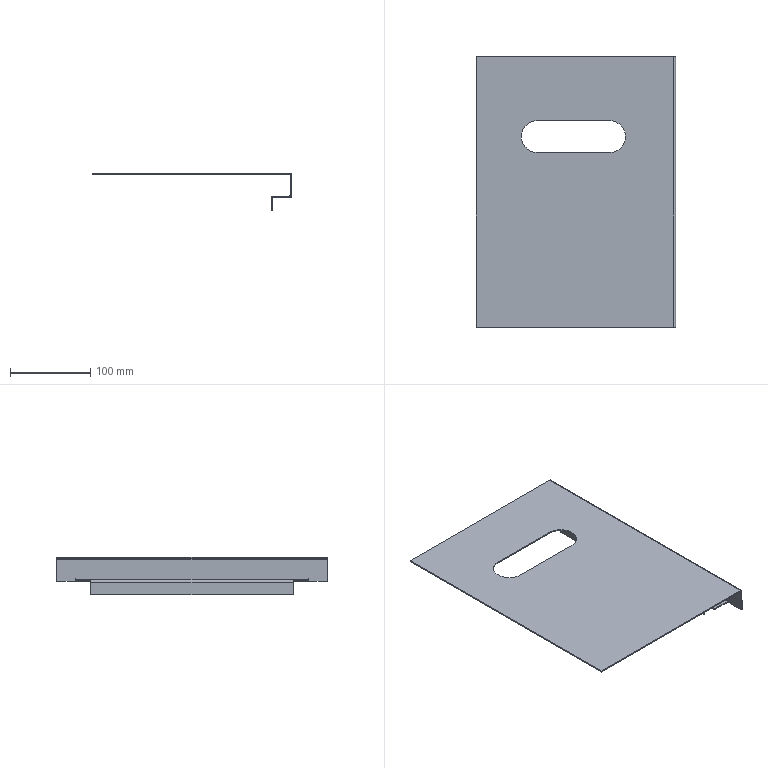Part | SolidWorks | features EdgeFlange 3, Cut 1, FlatPattern 1, SMBaseFlange 1, SheetMetal 1 | 1 solid | 51 faces | box 248.5 x 337 x 47 mm | volume 148406 mm3 | plane 42 | cylinder 9 | commonest cylinder face diameters 2 x3 5 x3 40 x3
STEP:
#1=CARTESIAN_POINT('',(56.,237.5,0.));
#2=VERTEX_POINT('',#1);
#3=CARTESIAN_POINT('',(76.,257.5,0.));
#4=VERTEX_POINT('',#3);
#5=CARTESIAN_POINT('',(76.,237.5,0.));
#6=DIRECTION('',(0.,0.,-1.));
#7=DIRECTION('',(-1.,0.,0.));
#8=AXIS2_PLACEMENT_3D('',#5,#6,#7);
#9=CIRCLE('',#8,20.);
#10=EDGE_CURVE('',#2,#4,#9,.T.);
#11=ORIENTED_EDGE('',*,*,#10,.F.);
#12=CARTESIAN_POINT('',(56.,237.5,-1.5));
#13=VERTEX_POINT('',#12);
#14=CARTESIAN_POINT('',(56.,237.5,0.));
#15=DIRECTION('',(0.,0.,-1.));
#16=VECTOR('',#15,1000.);
#17=LINE('',#14,#16);
#18=EDGE_CURVE('',#2,#13,#17,.T.);
#19=ORIENTED_EDGE('',*,*,#18,.T.);
#20=CARTESIAN_POINT('',(76.,257.5,-1.5));
#21=VERTEX_POINT('',#20);
#22=CARTESIAN_POINT('',(76.,237.5,-1.5));
#23=DIRECTION('',(0.,0.,-1.));
#24=DIRECTION('',(-1.,0.,0.));
#25=AXIS2_PLACEMENT_3D('',#22,#23,#24);
#26=CIRCLE('',#25,20.);
#27=EDGE_CURVE('',#13,#21,#26,.T.);
#28=ORIENTED_EDGE('',*,*,#27,.T.);
#29=CARTESIAN_POINT('',(76.,257.5,0.));
#30=DIRECTION('',(0.,0.,-1.));
#31=VECTOR('',#30,1000.);
#32=LINE('',#29,#31);
#33=EDGE_CURVE('',#4,#21,#32,.T.);
#34=ORIENTED_EDGE('',*,*,#33,.F.);
#35=EDGE_LOOP('',(#11,#19,#28,#34));
#36=FACE_OUTER_BOUND('',#35,.T.);
#37=CARTESIAN_POINT('',(76.,237.5,0.));
#38=DIRECTION('',(0.,0.,-1.));
#39=DIRECTION('',(-1.,0.,0.));
#40=AXIS2_PLACEMENT_3D('',#37,#38,#39);
#41=CYLINDRICAL_SURFACE('',#40,20.);
#42=ADVANCED_FACE('',(#36),#41,.F.);
#43=CARTESIAN_POINT('',(226.75,295.75,-30.));
#44=VERTEX_POINT('',#43);
#45=CARTESIAN_POINT('',(226.75,295.,-30.));
#46=VERTEX_POINT('',#45);
#47=CARTESIAN_POINT('',(226.75,295.75,-30.));
#48=DIRECTION('',(0.,-1.,0.));
#49=VECTOR('',#48,1000.);
#50=LINE('',#47,#49);
#51=EDGE_CURVE('',#44,#46,#50,.T.);
#52=ORIENTED_EDGE('',*,*,#51,.F.);
#53=CARTESIAN_POINT('',(223.5,295.75,-30.));
#54=VERTEX_POINT('',#53);
#55=CARTESIAN_POINT('',(223.5,295.75,-30.));
#56=DIRECTION('',(1.,0.,0.));
#57=VECTOR('',#56,1000.);
#58=LINE('',#55,#57);
#59=EDGE_CURVE('',#54,#44,#58,.T.);
#60=ORIENTED_EDGE('',*,*,#59,.F.);
#61=CARTESIAN_POINT('',(223.5,313.5,-30.));
#62=VERTEX_POINT('',#61);
#63=CARTESIAN_POINT('',(223.5,23.5,-30.));
#64=DIRECTION('',(0.,-1.,0.));
#65=VECTOR('',#64,1000.);
#66=LINE('',#63,#65);
#67=EDGE_CURVE('',#62,#54,#66,.T.);
#68=ORIENTED_EDGE('',*,*,#67,.F.);
#69=CARTESIAN_POINT('',(246.,313.5,-30.));
#70=VERTEX_POINT('',#69);
#71=CARTESIAN_POINT('',(223.5,313.5,-30.));
#72=DIRECTION('',(-1.,0.,0.));
#73=VECTOR('',#72,1000.);
#74=LINE('',#71,#73);
#75=EDGE_CURVE('',#70,#62,#74,.T.);
#76=ORIENTED_EDGE('',*,*,#75,.F.);
#77=CARTESIAN_POINT('',(246.,23.5,-30.));
#78=VERTEX_POINT('',#77);
#79=CARTESIAN_POINT('',(246.,0.,-30.));
#80=DIRECTION('',(0.,-1.,0.));
#81=VECTOR('',#80,1000.);
#82=LINE('',#79,#81);
#83=EDGE_CURVE('',#70,#78,#82,.T.);
#84=ORIENTED_EDGE('',*,*,#83,.T.);
#85=CARTESIAN_POINT('',(223.5,23.5,-30.));
#86=VERTEX_POINT('',#85);
#87=CARTESIAN_POINT('',(247.,23.5,-30.));
#88=DIRECTION('',(1.,0.,0.));
#89=VECTOR('',#88,1000.);
#90=LINE('',#87,#89);
#91=EDGE_CURVE('',#86,#78,#90,.T.);
#92=ORIENTED_EDGE('',*,*,#91,.F.);
#93=CARTESIAN_POINT('',(223.5,41.25,-30.));
#94=VERTEX_POINT('',#93);
#95=CARTESIAN_POINT('',(223.5,23.5,-30.));
#96=DIRECTION('',(0.,-1.,0.));
#97=VECTOR('',#96,1000.);
#98=LINE('',#95,#97);
#99=EDGE_CURVE('',#94,#86,#98,.T.);
#100=ORIENTED_EDGE('',*,*,#99,.F.);
#101=CARTESIAN_POINT('',(226.75,41.25,-30.));
#102=VERTEX_POINT('',#101);
#103=CARTESIAN_POINT('',(226.75,41.25,-30.));
#104=DIRECTION('',(-1.,0.,0.));
#105=VECTOR('',#104,1000.);
#106=LINE('',#103,#105);
#107=EDGE_CURVE('',#102,#94,#106,.T.);
#108=ORIENTED_EDGE('',*,*,#107,.F.);
#109=CARTESIAN_POINT('',(226.75,42.,-30.));
#110=VERTEX_POINT('',#109);
#111=CARTESIAN_POINT('',(226.75,42.,-30.));
#112=DIRECTION('',(0.,-1.,0.));
#113=VECTOR('',#112,1000.);
#114=LINE('',#111,#113);
#115=EDGE_CURVE('',#110,#102,#114,.T.);
#116=ORIENTED_EDGE('',*,*,#115,.F.);
#117=CARTESIAN_POINT('',(226.,42.,-30.));
#118=VERTEX_POINT('',#117);
#119=CARTESIAN_POINT('',(226.,42.,-30.));
#120=DIRECTION('',(1.,0.,0.));
#121=VECTOR('',#120,1000.);
#122=LINE('',#119,#121);
#123=EDGE_CURVE('',#118,#110,#122,.T.);
#124=ORIENTED_EDGE('',*,*,#123,.F.);
#125=CARTESIAN_POINT('',(226.,295.,-30.));
#126=VERTEX_POINT('',#125);
#127=CARTESIAN_POINT('',(226.,295.,-30.));
#128=DIRECTION('',(0.,-1.,0.));
#129=VECTOR('',#128,1000.);
#130=LINE('',#127,#129);
#131=EDGE_CURVE('',#126,#118,#130,.T.);
#132=ORIENTED_EDGE('',*,*,#131,.F.);
#133=CARTESIAN_POINT('',(226.75,295.,-30.));
#134=DIRECTION('',(-1.,0.,0.));
#135=VECTOR('',#134,1000.);
#136=LINE('',#133,#135);
#137=EDGE_CURVE('',#46,#126,#136,.T.);
#138=ORIENTED_EDGE('',*,*,#137,.F.);
#139=EDGE_LOOP('',(#52,#60,#68,#76,#84,#92,#100,#108,#116,#124,#132,#138));
#140=FACE_OUTER_BOUND('',#139,.T.);
#141=CARTESIAN_POINT('',(0.,0.,-30.));
#142=DIRECTION('',(0.,0.,-1.));
#143=DIRECTION('',(-1.,0.,0.));
#144=AXIS2_PLACEMENT_3D('',#141,#142,#143);
#145=PLANE('',#144);
#146=ADVANCED_FACE('',(#140),#145,.T.);
#147=CARTESIAN_POINT('',(226.75,295.75,-28.5));
#148=VERTEX_POINT('',#147);
#149=CARTESIAN_POINT('',(223.5,295.75,-28.5));
#150=VERTEX_POINT('',#149);
#151=CARTESIAN_POINT('',(0.,295.75,-28.5));
#152=DIRECTION('',(-1.,0.,0.));
#153=VECTOR('',#152,1000.);
#154=LINE('',#151,#153);
#155=EDGE_CURVE('',#148,#150,#154,.T.);
#156=ORIENTED_EDGE('',*,*,#155,.F.);
#157=CARTESIAN_POINT('',(226.75,295.,-28.5));
#158=VERTEX_POINT('',#157);
#159=CARTESIAN_POINT('',(226.75,0.,-28.5));
#160=DIRECTION('',(0.,1.,0.));
#161=VECTOR('',#160,1000.);
#162=LINE('',#159,#161);
#163=EDGE_CURVE('',#158,#148,#162,.T.);
#164=ORIENTED_EDGE('',*,*,#163,.F.);
#165=CARTESIAN_POINT('',(226.,295.,-28.5));
#166=VERTEX_POINT('',#165);
#167=CARTESIAN_POINT('',(0.,295.,-28.5));
#168=DIRECTION('',(1.,0.,0.));
#169=VECTOR('',#168,1000.);
#170=LINE('',#167,#169);
#171=EDGE_CURVE('',#166,#158,#170,.T.);
#172=ORIENTED_EDGE('',*,*,#171,.F.);
#173=CARTESIAN_POINT('',(226.,42.,-28.5));
#174=VERTEX_POINT('',#173);
#175=CARTESIAN_POINT('',(226.,295.,-28.5));
#176=DIRECTION('',(0.,-1.,0.));
#177=VECTOR('',#176,1000.);
#178=LINE('',#175,#177);
#179=EDGE_CURVE('',#166,#174,#178,.T.);
#180=ORIENTED_EDGE('',*,*,#179,.T.);
#181=CARTESIAN_POINT('',(226.75,42.,-28.5));
#182=VERTEX_POINT('',#181);
#183=CARTESIAN_POINT('',(0.,42.,-28.5));
#184=DIRECTION('',(-1.,0.,0.));
#185=VECTOR('',#184,1000.);
#186=LINE('',#183,#185);
#187=EDGE_CURVE('',#182,#174,#186,.T.);
#188=ORIENTED_EDGE('',*,*,#187,.F.);
#189=CARTESIAN_POINT('',(226.75,41.25,-28.5));
#190=VERTEX_POINT('',#189);
#191=CARTESIAN_POINT('',(226.75,0.,-28.5));
#192=DIRECTION('',(0.,1.,0.));
#193=VECTOR('',#192,1000.);
#194=LINE('',#191,#193);
#195=EDGE_CURVE('',#190,#182,#194,.T.);
#196=ORIENTED_EDGE('',*,*,#195,.F.);
#197=CARTESIAN_POINT('',(223.5,41.25,-28.5));
#198=VERTEX_POINT('',#197);
#199=CARTESIAN_POINT('',(0.,41.25,-28.5));
#200=DIRECTION('',(1.,0.,0.));
#201=VECTOR('',#200,1000.);
#202=LINE('',#199,#201);
#203=EDGE_CURVE('',#198,#190,#202,.T.);
#204=ORIENTED_EDGE('',*,*,#203,.F.);
#205=CARTESIAN_POINT('',(223.5,23.5,-28.5));
#206=VERTEX_POINT('',#205);
#207=CARTESIAN_POINT('',(223.5,0.,-28.5));
#208=DIRECTION('',(0.,-1.,0.));
#209=VECTOR('',#208,1000.);
#210=LINE('',#207,#209);
#211=EDGE_CURVE('',#198,#206,#210,.T.);
#212=ORIENTED_EDGE('',*,*,#211,.T.);
#213=CARTESIAN_POINT('',(246.,23.5,-28.5));
#214=VERTEX_POINT('',#213);
#215=CARTESIAN_POINT('',(0.,23.5,-28.5));
#216=DIRECTION('',(1.,0.,0.));
#217=VECTOR('',#216,1000.);
#218=LINE('',#215,#217);
#219=EDGE_CURVE('',#206,#214,#218,.T.);
#220=ORIENTED_EDGE('',*,*,#219,.T.);
#221=CARTESIAN_POINT('',(246.,313.5,-28.5));
#222=VERTEX_POINT('',#221);
#223=CARTESIAN_POINT('',(246.,313.5,-28.5));
#224=DIRECTION('',(0.,-1.,0.));
#225=VECTOR('',#224,1000.);
#226=LINE('',#223,#225);
#227=EDGE_CURVE('',#222,#214,#226,.T.);
#228=ORIENTED_EDGE('',*,*,#227,.F.);
#229=CARTESIAN_POINT('',(223.5,313.5,-28.5));
#230=VERTEX_POINT('',#229);
#231=CARTESIAN_POINT('',(0.,313.5,-28.5));
#232=DIRECTION('',(-1.,0.,0.));
#233=VECTOR('',#232,1000.);
#234=LINE('',#231,#233);
#235=EDGE_CURVE('',#222,#230,#234,.T.);
#236=ORIENTED_EDGE('',*,*,#235,.T.);
#237=CARTESIAN_POINT('',(223.5,0.,-28.5));
#238=DIRECTION('',(0.,-1.,0.));
#239=VECTOR('',#238,1000.);
#240=LINE('',#237,#239);
#241=EDGE_CURVE('',#230,#150,#240,.T.);
#242=ORIENTED_EDGE('',*,*,#241,.T.);
#243=EDGE_LOOP('',(#156,#164,#172,#180,#188,#196,#204,#212,#220,#228,#236,#242));
#244=FACE_OUTER_BOUND('',#243,.T.);
#245=CARTESIAN_POINT('',(0.,0.,-28.5));
#246=DIRECTION('',(0.,0.,-1.));
#247=DIRECTION('',(-1.,0.,0.));
#248=AXIS2_PLACEMENT_3D('',#245,#246,#247);
#249=PLANE('',#248);
#250=ADVANCED_FACE('',(#244),#249,.F.);
#251=ORIENTED_EDGE('',*,*,#67,.T.);
#252=CARTESIAN_POINT('',(223.5,295.75,-30.));
#253=DIRECTION('',(0.,0.,1.));
#254=VECTOR('',#253,1000.);
#255=LINE('',#252,#254);
#256=EDGE_CURVE('',#54,#150,#255,.T.);
#257=ORIENTED_EDGE('',*,*,#256,.T.);
#258=ORIENTED_EDGE('',*,*,#241,.F.);
#259=CARTESIAN_POINT('',(223.5,313.5,-30.));
#260=DIRECTION('',(0.,0.,1.));
#261=VECTOR('',#260,1000.);
#262=LINE('',#259,#261);
#263=EDGE_CURVE('',#62,#230,#262,.T.);
#264=ORIENTED_EDGE('',*,*,#263,.F.);
#265=EDGE_LOOP('',(#251,#257,#258,#264));
#266=FACE_OUTER_BOUND('',#265,.T.);
#267=CARTESIAN_POINT('',(223.5,23.5,-30.));
#268=DIRECTION('',(-1.,0.,0.));
#269=DIRECTION('',(0.,0.,1.));
#270=AXIS2_PLACEMENT_3D('',#267,#268,#269);
#271=PLANE('',#270);
#272=ADVANCED_FACE('',(#266),#271,.T.);
#273=ORIENTED_EDGE('',*,*,#211,.F.);
#274=CARTESIAN_POINT('',(223.5,41.25,-30.));
#275=DIRECTION('',(0.,0.,1.));
#276=VECTOR('',#275,1000.);
#277=LINE('',#274,#276);
#278=EDGE_CURVE('',#94,#198,#277,.T.);
#279=ORIENTED_EDGE('',*,*,#278,.F.);
#280=ORIENTED_EDGE('',*,*,#99,.T.);
#281=CARTESIAN_POINT('',(223.5,23.5,-30.));
#282=DIRECTION('',(0.,0.,1.));
#283=VECTOR('',#282,1000.);
#284=LINE('',#281,#283);
#285=EDGE_CURVE('',#86,#206,#284,.T.);
#286=ORIENTED_EDGE('',*,*,#285,.T.);
#287=EDGE_LOOP('',(#273,#279,#280,#286));
#288=FACE_OUTER_BOUND('',#287,.T.);
#289=CARTESIAN_POINT('',(223.5,23.5,-30.));
#290=DIRECTION('',(-1.,0.,0.));
#291=DIRECTION('',(0.,0.,1.));
#292=AXIS2_PLACEMENT_3D('',#289,#290,#291);
#293=PLANE('',#292);
#294=ADVANCED_FACE('',(#288),#293,.T.);
#295=CARTESIAN_POINT('',(248.5,22.75,-30.));
#296=VERTEX_POINT('',#295);
#297=CARTESIAN_POINT('',(248.5,0.,-30.));
#298=VERTEX_POINT('',#297);
#299=CARTESIAN_POINT('',(248.5,0.,-30.));
#300=DIRECTION('',(0.,-1.,0.));
#301=VECTOR('',#300,1000.);
#302=LINE('',#299,#301);
#303=EDGE_CURVE('',#296,#298,#302,.T.);
#304=ORIENTED_EDGE('',*,*,#303,.F.);
#305=CARTESIAN_POINT('',(248.5,22.75,-26.75));
#306=VERTEX_POINT('',#305);
#307=CARTESIAN_POINT('',(248.5,22.75,0.));
#308=DIRECTION('',(0.,0.,1.));
#309=VECTOR('',#308,1000.);
#310=LINE('',#307,#309);
#311=EDGE_CURVE('',#296,#306,#310,.T.);
#312=ORIENTED_EDGE('',*,*,#311,.T.);
#313=CARTESIAN_POINT('',(248.5,23.5,-26.75));
#314=VERTEX_POINT('',#313);
#315=CARTESIAN_POINT('',(248.5,0.,-26.75));
#316=DIRECTION('',(0.,1.,0.));
#317=VECTOR('',#316,1000.);
#318=LINE('',#315,#317);
#319=EDGE_CURVE('',#306,#314,#318,.T.);
#320=ORIENTED_EDGE('',*,*,#319,.T.);
#321=CARTESIAN_POINT('',(248.5,23.5,-27.5));
#322=VERTEX_POINT('',#321);
#323=CARTESIAN_POINT('',(248.5,23.5,0.));
#324=DIRECTION('',(0.,0.,-1.));
#325=VECTOR('',#324,1000.);
#326=LINE('',#323,#325);
#327=EDGE_CURVE('',#314,#322,#326,.T.);
#328=ORIENTED_EDGE('',*,*,#327,.T.);
#329=CARTESIAN_POINT('',(248.5,313.5,-27.5));
#330=VERTEX_POINT('',#329);
#331=CARTESIAN_POINT('',(248.5,23.5,-27.5));
#332=DIRECTION('',(0.,1.,0.));
#333=VECTOR('',#332,1000.);
#334=LINE('',#331,#333);
#335=EDGE_CURVE('',#322,#330,#334,.T.);
#336=ORIENTED_EDGE('',*,*,#335,.T.);
#337=CARTESIAN_POINT('',(248.5,313.5,-26.75));
#338=VERTEX_POINT('',#337);
#339=CARTESIAN_POINT('',(248.5,313.5,0.));
#340=DIRECTION('',(0.,0.,1.));
#341=VECTOR('',#340,1000.);
#342=LINE('',#339,#341);
#343=EDGE_CURVE('',#330,#338,#342,.T.);
#344=ORIENTED_EDGE('',*,*,#343,.T.);
#345=CARTESIAN_POINT('',(248.5,314.25,-26.75));
#346=VERTEX_POINT('',#345);
#347=CARTESIAN_POINT('',(248.5,0.,-26.75));
#348=DIRECTION('',(0.,1.,0.));
#349=VECTOR('',#348,1000.);
#350=LINE('',#347,#349);
#351=EDGE_CURVE('',#338,#346,#350,.T.);
#352=ORIENTED_EDGE('',*,*,#351,.T.);
#353=CARTESIAN_POINT('',(248.5,314.25,-30.));
#354=VERTEX_POINT('',#353);
#355=CARTESIAN_POINT('',(248.5,314.25,0.));
#356=DIRECTION('',(0.,0.,-1.));
#357=VECTOR('',#356,1000.);
#358=LINE('',#355,#357);
#359=EDGE_CURVE('',#346,#354,#358,.T.);
#360=ORIENTED_EDGE('',*,*,#359,.T.);
#361=CARTESIAN_POINT('',(248.5,337.,-30.));
#362=VERTEX_POINT('',#361);
#363=CARTESIAN_POINT('',(248.5,0.,-30.));
#364=DIRECTION('',(0.,-1.,0.));
#365=VECTOR('',#364,1000.);
#366=LINE('',#363,#365);
#367=EDGE_CURVE('',#362,#354,#366,.T.);
#368=ORIENTED_EDGE('',*,*,#367,.F.);
#369=CARTESIAN_POINT('',(248.5,337.,-2.5));
#370=VERTEX_POINT('',#369);
#371=CARTESIAN_POINT('',(248.5,337.,-30.));
#372=DIRECTION('',(0.,0.,-1.));
#373=VECTOR('',#372,1000.);
#374=LINE('',#371,#373);
#375=EDGE_CURVE('',#370,#362,#374,.T.);
#376=ORIENTED_EDGE('',*,*,#375,.F.);
#377=CARTESIAN_POINT('',(248.5,0.,-2.5));
#378=VERTEX_POINT('',#377);
#379=CARTESIAN_POINT('',(248.5,0.,-2.5));
#380=DIRECTION('',(0.,-1.,0.));
#381=VECTOR('',#380,1000.);
#382=LINE('',#379,#381);
#383=EDGE_CURVE('',#370,#378,#382,.T.);
#384=ORIENTED_EDGE('',*,*,#383,.T.);
#385=CARTESIAN_POINT('',(248.5,0.,-1.5));
#386=DIRECTION('',(0.,0.,1.));
#387=VECTOR('',#386,1000.);
#388=LINE('',#385,#387);
#389=EDGE_CURVE('',#298,#378,#388,.T.);
#390=ORIENTED_EDGE('',*,*,#389,.F.);
#391=EDGE_LOOP('',(#304,#312,#320,#328,#336,#344,#352,#360,#368,#376,#384,#390));
#392=FACE_OUTER_BOUND('',#391,.T.);
#393=CARTESIAN_POINT('',(248.5,0.,0.));
#394=DIRECTION('',(1.,0.,0.));
#395=DIRECTION('',(0.,0.,-1.));
#396=AXIS2_PLACEMENT_3D('',#393,#394,#395);
#397=PLANE('',#396);
#398=ADVANCED_FACE('',(#392),#397,.T.);
#399=CARTESIAN_POINT('',(247.,22.75,-30.));
#400=VERTEX_POINT('',#399);
#401=CARTESIAN_POINT('',(247.,22.75,-26.75));
#402=VERTEX_POINT('',#401);
#403=CARTESIAN_POINT('',(247.,22.75,-30.));
#404=DIRECTION('',(0.,0.,1.));
#405=VECTOR('',#404,1000.);
#406=LINE('',#403,#405);
#407=EDGE_CURVE('',#400,#402,#406,.T.);
#408=ORIENTED_EDGE('',*,*,#407,.F.);
#409=CARTESIAN_POINT('',(247.,0.,-30.));
#410=VERTEX_POINT('',#409);
#411=CARTESIAN_POINT('',(247.,0.,-30.));
#412=DIRECTION('',(0.,-1.,0.));
#413=VECTOR('',#412,1000.);
#414=LINE('',#411,#413);
#415=EDGE_CURVE('',#400,#410,#414,.T.);
#416=ORIENTED_EDGE('',*,*,#415,.T.);
#417=CARTESIAN_POINT('',(247.,0.,-2.5));
#418=VERTEX_POINT('',#417);
#419=CARTESIAN_POINT('',(247.,0.,0.));
#420=DIRECTION('',(0.,0.,1.));
#421=VECTOR('',#420,1000.);
#422=LINE('',#419,#421);
#423=EDGE_CURVE('',#410,#418,#422,.T.);
#424=ORIENTED_EDGE('',*,*,#423,.T.);
#425=CARTESIAN_POINT('',(247.,337.,-2.5));
#426=VERTEX_POINT('',#425);
#427=CARTESIAN_POINT('',(247.,337.,-2.5));
#428=DIRECTION('',(0.,-1.,0.));
#429=VECTOR('',#428,1000.);
#430=LINE('',#427,#429);
#431=EDGE_CURVE('',#426,#418,#430,.T.);
#432=ORIENTED_EDGE('',*,*,#431,.F.);
#433=CARTESIAN_POINT('',(247.,337.,-30.));
#434=VERTEX_POINT('',#433);
#435=CARTESIAN_POINT('',(247.,337.,0.));
#436=DIRECTION('',(0.,0.,-1.));
#437=VECTOR('',#436,1000.);
#438=LINE('',#435,#437);
#439=EDGE_CURVE('',#426,#434,#438,.T.);
#440=ORIENTED_EDGE('',*,*,#439,.T.);
#441=CARTESIAN_POINT('',(247.,314.25,-30.));
#442=VERTEX_POINT('',#441);
#443=CARTESIAN_POINT('',(247.,0.,-30.));
#444=DIRECTION('',(0.,-1.,0.));
#445=VECTOR('',#444,1000.);
#446=LINE('',#443,#445);
#447=EDGE_CURVE('',#434,#442,#446,.T.);
#448=ORIENTED_EDGE('',*,*,#447,.T.);
#449=CARTESIAN_POINT('',(247.,314.25,-26.75));
#450=VERTEX_POINT('',#449);
#451=CARTESIAN_POINT('',(247.,314.25,-26.75));
#452=DIRECTION('',(0.,0.,-1.));
#453=VECTOR('',#452,1000.);
#454=LINE('',#451,#453);
#455=EDGE_CURVE('',#450,#442,#454,.T.);
#456=ORIENTED_EDGE('',*,*,#455,.F.);
#457=CARTESIAN_POINT('',(247.,313.5,-26.75));
#458=VERTEX_POINT('',#457);
#459=CARTESIAN_POINT('',(247.,313.5,-26.75));
#460=DIRECTION('',(0.,1.,0.));
#461=VECTOR('',#460,1000.);
#462=LINE('',#459,#461);
#463=EDGE_CURVE('',#458,#450,#462,.T.);
#464=ORIENTED_EDGE('',*,*,#463,.F.);
#465=CARTESIAN_POINT('',(247.,313.5,-27.5));
#466=VERTEX_POINT('',#465);
#467=CARTESIAN_POINT('',(247.,313.5,-27.5));
#468=DIRECTION('',(0.,0.,1.));
#469=VECTOR('',#468,1000.);
#470=LINE('',#467,#469);
#471=EDGE_CURVE('',#466,#458,#470,.T.);
#472=ORIENTED_EDGE('',*,*,#471,.F.);
#473=CARTESIAN_POINT('',(247.,23.5,-27.5));
#474=VERTEX_POINT('',#473);
#475=CARTESIAN_POINT('',(247.,23.5,-27.5));
#476=DIRECTION('',(0.,1.,0.));
#477=VECTOR('',#476,1000.);
#478=LINE('',#475,#477);
#479=EDGE_CURVE('',#474,#466,#478,.T.);
#480=ORIENTED_EDGE('',*,*,#479,.F.);
#481=CARTESIAN_POINT('',(247.,23.5,-26.75));
#482=VERTEX_POINT('',#481);
#483=CARTESIAN_POINT('',(247.,23.5,-26.75));
#484=DIRECTION('',(0.,0.,-1.));
#485=VECTOR('',#484,1000.);
#486=LINE('',#483,#485);
#487=EDGE_CURVE('',#482,#474,#486,.T.);
#488=ORIENTED_EDGE('',*,*,#487,.F.);
#489=CARTESIAN_POINT('',(247.,22.75,-26.75));
#490=DIRECTION('',(0.,1.,0.));
#491=VECTOR('',#490,1000.);
#492=LINE('',#489,#491);
#493=EDGE_CURVE('',#402,#482,#492,.T.);
#494=ORIENTED_EDGE('',*,*,#493,.F.);
#495=EDGE_LOOP('',(#408,#416,#424,#432,#440,#448,#456,#464,#472,#480,#488,#494));
#496=FACE_OUTER_BOUND('',#495,.T.);
#497=CARTESIAN_POINT('',(247.,0.,0.));
#498=DIRECTION('',(1.,0.,0.));
#499=DIRECTION('',(0.,0.,-1.));
#500=AXIS2_PLACEMENT_3D('',#497,#498,#499);
#501=PLANE('',#500);
#502=ADVANCED_FACE('',(#496),#501,.F.);
#503=ORIENTED_EDGE('',*,*,#415,.F.);
#504=CARTESIAN_POINT('',(247.,22.75,-30.));
#505=DIRECTION('',(1.,0.,0.));
#506=VECTOR('',#505,1000.);
#507=LINE('',#504,#506);
#508=EDGE_CURVE('',#400,#296,#507,.T.);
#509=ORIENTED_EDGE('',*,*,#508,.T.);
#510=ORIENTED_EDGE('',*,*,#303,.T.);
#511=CARTESIAN_POINT('',(248.5,0.,-30.));
#512=DIRECTION('',(-1.,0.,0.));
#513=VECTOR('',#512,1000.);
#514=LINE('',#511,#513);
#515=EDGE_CURVE('',#298,#410,#514,.T.);
#516=ORIENTED_EDGE('',*,*,#515,.T.);
#517=EDGE_LOOP('',(#503,#509,#510,#516));
#518=FACE_OUTER_BOUND('',#517,.T.);
#519=CARTESIAN_POINT('',(248.5,0.,-30.));
#520=DIRECTION('',(0.,0.,-1.));
#521=DIRECTION('',(-1.,0.,0.));
#522=AXIS2_PLACEMENT_3D('',#519,#520,#521);
#523=PLANE('',#522);
#524=ADVANCED_FACE('',(#518),#523,.T.);
#525=ORIENTED_EDGE('',*,*,#367,.T.);
#526=CARTESIAN_POINT('',(247.,314.25,-30.));
#527=DIRECTION('',(1.,0.,0.));
#528=VECTOR('',#527,1000.);
#529=LINE('',#526,#528);
#530=EDGE_CURVE('',#442,#354,#529,.T.);
#531=ORIENTED_EDGE('',*,*,#530,.F.);
#532=ORIENTED_EDGE('',*,*,#447,.F.);
#533=CARTESIAN_POINT('',(248.5,337.,-30.));
#534=DIRECTION('',(-1.,0.,0.));
#535=VECTOR('',#534,1000.);
#536=LINE('',#533,#535);
#537=EDGE_CURVE('',#362,#434,#536,.T.);
#538=ORIENTED_EDGE('',*,*,#537,.F.);
#539=EDGE_LOOP('',(#525,#531,#532,#538));
#540=FACE_OUTER_BOUND('',#539,.T.);
#541=CARTESIAN_POINT('',(248.5,0.,-30.));
#542=DIRECTION('',(0.,0.,-1.));
#543=DIRECTION('',(-1.,0.,0.));
#544=AXIS2_PLACEMENT_3D('',#541,#542,#543);
#545=PLANE('',#544);
#546=ADVANCED_FACE('',(#540),#545,.T.);
#547=CARTESIAN_POINT('',(0.,0.,-1.5));
#548=VERTEX_POINT('',#547);
#549=CARTESIAN_POINT('',(246.,0.,-1.5));
#550=VERTEX_POINT('',#549);
#551=CARTESIAN_POINT('',(0.,0.,-1.5));
#552=DIRECTION('',(1.,0.,0.));
#553=VECTOR('',#552,1000.);
#554=LINE('',#551,#553);
#555=EDGE_CURVE('',#548,#550,#554,.T.);
#556=ORIENTED_EDGE('',*,*,#555,.T.);
#557=CARTESIAN_POINT('',(246.,0.,0.));
#558=VERTEX_POINT('',#557);
#559=CARTESIAN_POINT('',(246.,0.,-1.5));
#560=DIRECTION('',(0.,0.,1.));
#561=VECTOR('',#560,1000.);
#562=LINE('',#559,#561);
#563=EDGE_CURVE('',#550,#558,#562,.T.);
#564=ORIENTED_EDGE('',*,*,#563,.T.);
#565=CARTESIAN_POINT('',(0.,0.,0.));
#566=VERTEX_POINT('',#565);
#567=CARTESIAN_POINT('',(0.,0.,0.));
#568=DIRECTION('',(1.,0.,0.));
#569=VECTOR('',#568,1000.);
#570=LINE('',#567,#569);
#571=EDGE_CURVE('',#566,#558,#570,.T.);
#572=ORIENTED_EDGE('',*,*,#571,.F.);
#573=CARTESIAN_POINT('',(0.,0.,-1.5));
#574=DIRECTION('',(0.,0.,1.));
#575=VECTOR('',#574,1000.);
#576=LINE('',#573,#575);
#577=EDGE_CURVE('',#548,#566,#576,.T.);
#578=ORIENTED_EDGE('',*,*,#577,.F.);
#579=EDGE_LOOP('',(#556,#564,#572,#578));
#580=FACE_OUTER_BOUND('',#579,.T.);
#581=CARTESIAN_POINT('',(0.,0.,-1.5));
#582=DIRECTION('',(0.,-1.,0.));
#583=DIRECTION('',(0.,0.,-1.));
#584=AXIS2_PLACEMENT_3D('',#581,#582,#583);
#585=PLANE('',#584);
#586=ADVANCED_FACE('',(#580),#585,.T.);
#587=CARTESIAN_POINT('',(76.,217.5,-1.5));
#588=VERTEX_POINT('',#587);
#589=CARTESIAN_POINT('',(76.,237.5,-1.5));
#590=DIRECTION('',(0.,0.,-1.));
#591=DIRECTION('',(-1.,0.,0.));
#592=AXIS2_PLACEMENT_3D('',#589,#590,#591);
#593=CIRCLE('',#592,20.);
#594=EDGE_CURVE('',#588,#13,#593,.T.);
#595=ORIENTED_EDGE('',*,*,#594,.F.);
#596=CARTESIAN_POINT('',(166.,217.5,-1.5));
#597=VERTEX_POINT('',#596);
#598=CARTESIAN_POINT('',(76.,217.5,-1.5));
#599=DIRECTION('',(-1.,0.,0.));
#600=VECTOR('',#599,1000.);
#601=LINE('',#598,#600);
#602=EDGE_CURVE('',#597,#588,#601,.T.);
#603=ORIENTED_EDGE('',*,*,#602,.F.);
#604=CARTESIAN_POINT('',(166.,257.5,-1.5));
#605=VERTEX_POINT('',#604);
#606=CARTESIAN_POINT('',(166.,237.5,-1.5));
#607=DIRECTION('',(0.,0.,-1.));
#608=DIRECTION('',(-1.,0.,0.));
#609=AXIS2_PLACEMENT_3D('',#606,#607,#608);
#610=CIRCLE('',#609,20.);
#611=EDGE_CURVE('',#605,#597,#610,.T.);
#612=ORIENTED_EDGE('',*,*,#611,.F.);
#613=CARTESIAN_POINT('',(76.,257.5,-1.5));
#614=DIRECTION('',(1.,0.,0.));
#615=VECTOR('',#614,1000.);
#616=LINE('',#613,#615);
#617=EDGE_CURVE('',#21,#605,#616,.T.);
#618=ORIENTED_EDGE('',*,*,#617,.F.);
#619=ORIENTED_EDGE('',*,*,#27,.F.);
#620=EDGE_LOOP('',(#595,#603,#612,#618,#619));
#621=FACE_BOUND('',#620,.T.);
#622=CARTESIAN_POINT('',(246.,337.,-1.5));
#623=VERTEX_POINT('',#622);
#624=CARTESIAN_POINT('',(0.,337.,-1.5));
#625=VERTEX_POINT('',#624);
#626=CARTESIAN_POINT('',(0.,337.,-1.5));
#627=DIRECTION('',(-1.,0.,0.));
#628=VECTOR('',#627,1000.);
#629=LINE('',#626,#628);
#630=EDGE_CURVE('',#623,#625,#629,.T.);
#631=ORIENTED_EDGE('',*,*,#630,.F.);
#632=CARTESIAN_POINT('',(246.,0.,-1.5));
#633=DIRECTION('',(0.,1.,0.));
#634=VECTOR('',#633,1000.);
#635=LINE('',#632,#634);
#636=EDGE_CURVE('',#550,#623,#635,.T.);
#637=ORIENTED_EDGE('',*,*,#636,.F.);
#638=ORIENTED_EDGE('',*,*,#555,.F.);
#639=CARTESIAN_POINT('',(0.,0.,-1.5));
#640=DIRECTION('',(0.,-1.,0.));
#641=VECTOR('',#640,1000.);
#642=LINE('',#639,#641);
#643=EDGE_CURVE('',#625,#548,#642,.T.);
#644=ORIENTED_EDGE('',*,*,#643,.F.);
#645=EDGE_LOOP('',(#631,#637,#638,#644));
#646=FACE_OUTER_BOUND('',#645,.T.);
#647=CARTESIAN_POINT('',(0.,0.,-1.5));
#648=DIRECTION('',(0.,0.,-1.));
#649=DIRECTION('',(-1.,0.,0.));
#650=AXIS2_PLACEMENT_3D('',#647,#648,#649);
#651=PLANE('',#650);
#652=ADVANCED_FACE('',(#621,#646),#651,.T.);
#653=CARTESIAN_POINT('',(166.,217.5,0.));
#654=VERTEX_POINT('',#653);
#655=CARTESIAN_POINT('',(76.,217.5,0.));
#656=VERTEX_POINT('',#655);
#657=CARTESIAN_POINT('',(76.,217.5,0.));
#658=DIRECTION('',(-1.,0.,0.));
#659=VECTOR('',#658,1000.);
#660=LINE('',#657,#659);
#661=EDGE_CURVE('',#654,#656,#660,.T.);
#662=ORIENTED_EDGE('',*,*,#661,.T.);
#663=CARTESIAN_POINT('',(76.,237.5,0.));
#664=DIRECTION('',(0.,0.,-1.));
#665=DIRECTION('',(-1.,0.,0.));
#666=AXIS2_PLACEMENT_3D('',#663,#664,#665);
#667=CIRCLE('',#666,20.);
#668=EDGE_CURVE('',#656,#2,#667,.T.);
#669=ORIENTED_EDGE('',*,*,#668,.T.);
#670=ORIENTED_EDGE('',*,*,#10,.T.);
#671=CARTESIAN_POINT('',(166.,257.5,0.));
#672=VERTEX_POINT('',#671);
#673=CARTESIAN_POINT('',(76.,257.5,0.));
#674=DIRECTION('',(1.,0.,0.));
#675=VECTOR('',#674,1000.);
#676=LINE('',#673,#675);
#677=EDGE_CURVE('',#4,#672,#676,.T.);
#678=ORIENTED_EDGE('',*,*,#677,.T.);
#679=CARTESIAN_POINT('',(166.,237.5,0.));
#680=DIRECTION('',(0.,0.,-1.));
#681=DIRECTION('',(-1.,0.,0.));
#682=AXIS2_PLACEMENT_3D('',#679,#680,#681);
#683=CIRCLE('',#682,20.);
#684=EDGE_CURVE('',#672,#654,#683,.T.);
#685=ORIENTED_EDGE('',*,*,#684,.T.);
#686=EDGE_LOOP('',(#662,#669,#670,#678,#685));
#687=FACE_BOUND('',#686,.T.);
#688=CARTESIAN_POINT('',(246.,337.,0.));
#689=VERTEX_POINT('',#688);
#690=CARTESIAN_POINT('',(246.,0.,0.));
#691=DIRECTION('',(0.,1.,0.));
#692=VECTOR('',#691,1000.);
#693=LINE('',#690,#692);
#694=EDGE_CURVE('',#558,#689,#693,.T.);
#695=ORIENTED_EDGE('',*,*,#694,.T.);
#696=CARTESIAN_POINT('',(0.,337.,0.));
#697=VERTEX_POINT('',#696);
#698=CARTESIAN_POINT('',(0.,337.,0.));
#699=DIRECTION('',(-1.,0.,0.));
#700=VECTOR('',#699,1000.);
#701=LINE('',#698,#700);
#702=EDGE_CURVE('',#689,#697,#701,.T.);
#703=ORIENTED_EDGE('',*,*,#702,.T.);
#704=CARTESIAN_POINT('',(0.,0.,0.));
#705=DIRECTION('',(0.,-1.,0.));
#706=VECTOR('',#705,1000.);
#707=LINE('',#704,#706);
#708=EDGE_CURVE('',#697,#566,#707,.T.);
#709=ORIENTED_EDGE('',*,*,#708,.T.);
#710=ORIENTED_EDGE('',*,*,#571,.T.);
#711=EDGE_LOOP('',(#695,#703,#709,#710));
#712=FACE_OUTER_BOUND('',#711,.T.);
#713=CARTESIAN_POINT('',(0.,0.,0.));
#714=DIRECTION('',(0.,0.,-1.));
#715=DIRECTION('',(-1.,0.,0.));
#716=AXIS2_PLACEMENT_3D('',#713,#714,#715);
#717=PLANE('',#716);
#718=ADVANCED_FACE('',(#687,#712),#717,.F.);
#719=ORIENTED_EDGE('',*,*,#708,.F.);
#720=CARTESIAN_POINT('',(0.,337.,-1.5));
#721=DIRECTION('',(0.,0.,1.));
#722=VECTOR('',#721,1000.);
#723=LINE('',#720,#722);
#724=EDGE_CURVE('',#625,#697,#723,.T.);
#725=ORIENTED_EDGE('',*,*,#724,.F.);
#726=ORIENTED_EDGE('',*,*,#643,.T.);
#727=ORIENTED_EDGE('',*,*,#577,.T.);
#728=EDGE_LOOP('',(#719,#725,#726,#727));
#729=FACE_OUTER_BOUND('',#728,.T.);
#730=CARTESIAN_POINT('',(0.,0.,-1.5));
#731=DIRECTION('',(-1.,0.,0.));
#732=DIRECTION('',(0.,0.,1.));
#733=AXIS2_PLACEMENT_3D('',#730,#731,#732);
#734=PLANE('',#733);
#735=ADVANCED_FACE('',(#729),#734,.T.);
#736=CARTESIAN_POINT('',(246.,337.,-1.5));
#737=DIRECTION('',(0.,0.,1.));
#738=VECTOR('',#737,1000.);
#739=LINE('',#736,#738);
#740=EDGE_CURVE('',#623,#689,#739,.T.);
#741=ORIENTED_EDGE('',*,*,#740,.F.);
#742=ORIENTED_EDGE('',*,*,#630,.T.);
#743=ORIENTED_EDGE('',*,*,#724,.T.);
#744=ORIENTED_EDGE('',*,*,#702,.F.);
#745=EDGE_LOOP('',(#741,#742,#743,#744));
#746=FACE_OUTER_BOUND('',#745,.T.);
#747=CARTESIAN_POINT('',(0.,337.,-1.5));
#748=DIRECTION('',(0.,1.,0.));
#749=DIRECTION('',(0.,0.,1.));
#750=AXIS2_PLACEMENT_3D('',#747,#748,#749);
#751=PLANE('',#750);
#752=ADVANCED_FACE('',(#746),#751,.T.);
#753=CARTESIAN_POINT('',(248.5,337.,-2.5));
#754=DIRECTION('',(1.,0.,0.));
#755=VECTOR('',#754,1000.);
#756=LINE('',#753,#755);
#757=EDGE_CURVE('',#426,#370,#756,.T.);
#758=ORIENTED_EDGE('',*,*,#757,.F.);
#759=CARTESIAN_POINT('',(246.,337.,-2.5));
#760=DIRECTION('',(0.,1.,0.));
#761=DIRECTION('',(0.,0.,-1.));
#762=AXIS2_PLACEMENT_3D('',#759,#760,#761);
#763=CIRCLE('',#762,1.);
#764=EDGE_CURVE('',#623,#426,#763,.T.);
#765=ORIENTED_EDGE('',*,*,#764,.F.);
#766=ORIENTED_EDGE('',*,*,#740,.T.);
#767=CARTESIAN_POINT('',(246.,337.,-2.5));
#768=DIRECTION('',(0.,1.,0.));
#769=DIRECTION('',(0.,0.,-1.));
#770=AXIS2_PLACEMENT_3D('',#767,#768,#769);
#771=CIRCLE('',#770,2.5);
#772=EDGE_CURVE('',#689,#370,#771,.T.);
#773=ORIENTED_EDGE('',*,*,#772,.T.);
#774=EDGE_LOOP('',(#758,#765,#766,#773));
#775=FACE_OUTER_BOUND('',#774,.T.);
#776=CARTESIAN_POINT('',(246.,337.,-2.5));
#777=DIRECTION('',(0.,1.,0.));
#778=DIRECTION('',(0.,0.,1.));
#779=AXIS2_PLACEMENT_3D('',#776,#777,#778);
#780=PLANE('',#779);
#781=ADVANCED_FACE('',(#775),#780,.T.);
#782=CARTESIAN_POINT('',(246.,0.,-2.5));
#783=DIRECTION('',(0.,-1.,0.));
#784=DIRECTION('',(0.,0.,-1.));
#785=AXIS2_PLACEMENT_3D('',#782,#783,#784);
#786=CIRCLE('',#785,1.);
#787=EDGE_CURVE('',#418,#550,#786,.T.);
#788=ORIENTED_EDGE('',*,*,#787,.F.);
#789=CARTESIAN_POINT('',(247.,0.,-2.5));
#790=DIRECTION('',(1.,0.,0.));
#791=VECTOR('',#790,1000.);
#792=LINE('',#789,#791);
#793=EDGE_CURVE('',#418,#378,#792,.T.);
#794=ORIENTED_EDGE('',*,*,#793,.T.);
#795=CARTESIAN_POINT('',(246.,0.,-2.5));
#796=DIRECTION('',(0.,-1.,0.));
#797=DIRECTION('',(0.,0.,-1.));
#798=AXIS2_PLACEMENT_3D('',#795,#796,#797);
#799=CIRCLE('',#798,2.5);
#800=EDGE_CURVE('',#378,#558,#799,.T.);
#801=ORIENTED_EDGE('',*,*,#800,.T.);
#802=ORIENTED_EDGE('',*,*,#563,.F.);
#803=EDGE_LOOP('',(#788,#794,#801,#802));
#804=FACE_OUTER_BOUND('',#803,.T.);
#805=CARTESIAN_POINT('',(246.,0.,-2.5));
#806=DIRECTION('',(0.,1.,0.));
#807=DIRECTION('',(0.,0.,1.));
#808=AXIS2_PLACEMENT_3D('',#805,#806,#807);
#809=PLANE('',#808);
#810=ADVANCED_FACE('',(#804),#809,.F.);
#811=ORIENTED_EDGE('',*,*,#694,.F.);
#812=ORIENTED_EDGE('',*,*,#800,.F.);
#813=ORIENTED_EDGE('',*,*,#383,.F.);
#814=ORIENTED_EDGE('',*,*,#772,.F.);
#815=EDGE_LOOP('',(#811,#812,#813,#814));
#816=FACE_OUTER_BOUND('',#815,.T.);
#817=CARTESIAN_POINT('',(246.,0.,-2.5));
#818=DIRECTION('',(0.,-1.,0.));
#819=DIRECTION('',(1.,0.,0.));
#820=AXIS2_PLACEMENT_3D('',#817,#818,#819);
#821=CYLINDRICAL_SURFACE('',#820,2.5);
#822=ADVANCED_FACE('',(#816),#821,.T.);
#823=ORIENTED_EDGE('',*,*,#636,.T.);
#824=ORIENTED_EDGE('',*,*,#764,.T.);
#825=ORIENTED_EDGE('',*,*,#431,.T.);
#826=ORIENTED_EDGE('',*,*,#787,.T.);
#827=EDGE_LOOP('',(#823,#824,#825,#826));
#828=FACE_OUTER_BOUND('',#827,.T.);
#829=CARTESIAN_POINT('',(246.,0.,-2.5));
#830=DIRECTION('',(0.,-1.,0.));
#831=DIRECTION('',(1.,0.,0.));
#832=AXIS2_PLACEMENT_3D('',#829,#830,#831);
#833=CYLINDRICAL_SURFACE('',#832,1.);
#834=ADVANCED_FACE('',(#828),#833,.F.);
#835=ORIENTED_EDGE('',*,*,#389,.T.);
#836=ORIENTED_EDGE('',*,*,#793,.F.);
#837=ORIENTED_EDGE('',*,*,#423,.F.);
#838=ORIENTED_EDGE('',*,*,#515,.F.);
#839=EDGE_LOOP('',(#835,#836,#837,#838));
#840=FACE_OUTER_BOUND('',#839,.T.);
#841=CARTESIAN_POINT('',(248.5,0.,-1.5));
#842=DIRECTION('',(0.,-1.,0.));
#843=DIRECTION('',(0.,0.,-1.));
#844=AXIS2_PLACEMENT_3D('',#841,#842,#843);
#845=PLANE('',#844);
#846=ADVANCED_FACE('',(#840),#845,.T.);
#847=ORIENTED_EDGE('',*,*,#439,.F.);
#848=ORIENTED_EDGE('',*,*,#757,.T.);
#849=ORIENTED_EDGE('',*,*,#375,.T.);
#850=ORIENTED_EDGE('',*,*,#537,.T.);
#851=EDGE_LOOP('',(#847,#848,#849,#850));
#852=FACE_OUTER_BOUND('',#851,.T.);
#853=CARTESIAN_POINT('',(248.5,337.,-30.));
#854=DIRECTION('',(0.,1.,0.));
#855=DIRECTION('',(0.,0.,1.));
#856=AXIS2_PLACEMENT_3D('',#853,#854,#855);
#857=PLANE('',#856);
#858=ADVANCED_FACE('',(#852),#857,.T.);
#859=ORIENTED_EDGE('',*,*,#311,.F.);
#860=ORIENTED_EDGE('',*,*,#508,.F.);
#861=ORIENTED_EDGE('',*,*,#407,.T.);
#862=CARTESIAN_POINT('',(247.,22.75,-26.75));
#863=DIRECTION('',(1.,0.,0.));
#864=VECTOR('',#863,1000.);
#865=LINE('',#862,#864);
#866=EDGE_CURVE('',#402,#306,#865,.T.);
#867=ORIENTED_EDGE('',*,*,#866,.T.);
#868=EDGE_LOOP('',(#859,#860,#861,#867));
#869=FACE_OUTER_BOUND('',#868,.T.);
#870=CARTESIAN_POINT('',(247.,22.75,-30.));
#871=DIRECTION('',(0.,1.,0.));
#872=DIRECTION('',(0.,0.,1.));
#873=AXIS2_PLACEMENT_3D('',#870,#871,#872);
#874=PLANE('',#873);
#875=ADVANCED_FACE('',(#869),#874,.T.);
#876=ORIENTED_EDGE('',*,*,#319,.F.);
#877=ORIENTED_EDGE('',*,*,#866,.F.);
#878=ORIENTED_EDGE('',*,*,#493,.T.);
#879=CARTESIAN_POINT('',(247.,23.5,-26.75));
#880=DIRECTION('',(1.,0.,0.));
#881=VECTOR('',#880,1000.);
#882=LINE('',#879,#881);
#883=EDGE_CURVE('',#482,#314,#882,.T.);
#884=ORIENTED_EDGE('',*,*,#883,.T.);
#885=EDGE_LOOP('',(#876,#877,#878,#884));
#886=FACE_OUTER_BOUND('',#885,.T.);
#887=CARTESIAN_POINT('',(247.,22.75,-26.75));
#888=DIRECTION('',(0.,0.,-1.));
#889=DIRECTION('',(-1.,0.,0.));
#890=AXIS2_PLACEMENT_3D('',#887,#888,#889);
#891=PLANE('',#890);
#892=ADVANCED_FACE('',(#886),#891,.T.);
#893=ORIENTED_EDGE('',*,*,#327,.F.);
#894=ORIENTED_EDGE('',*,*,#883,.F.);
#895=ORIENTED_EDGE('',*,*,#487,.T.);
#896=CARTESIAN_POINT('',(247.,23.5,-27.5));
#897=DIRECTION('',(1.,0.,0.));
#898=VECTOR('',#897,1000.);
#899=LINE('',#896,#898);
#900=EDGE_CURVE('',#474,#322,#899,.T.);
#901=ORIENTED_EDGE('',*,*,#900,.T.);
#902=EDGE_LOOP('',(#893,#894,#895,#901));
#903=FACE_OUTER_BOUND('',#902,.T.);
#904=CARTESIAN_POINT('',(247.,23.5,-26.75));
#905=DIRECTION('',(0.,-1.,0.));
#906=DIRECTION('',(0.,0.,-1.));
#907=AXIS2_PLACEMENT_3D('',#904,#905,#906);
#908=PLANE('',#907);
#909=ADVANCED_FACE('',(#903),#908,.T.);
#910=ORIENTED_EDGE('',*,*,#343,.F.);
#911=CARTESIAN_POINT('',(247.,313.5,-27.5));
#912=DIRECTION('',(1.,0.,0.));
#913=VECTOR('',#912,1000.);
#914=LINE('',#911,#913);
#915=EDGE_CURVE('',#466,#330,#914,.T.);
#916=ORIENTED_EDGE('',*,*,#915,.F.);
#917=ORIENTED_EDGE('',*,*,#471,.T.);
#918=CARTESIAN_POINT('',(247.,313.5,-26.75));
#919=DIRECTION('',(1.,0.,0.));
#920=VECTOR('',#919,1000.);
#921=LINE('',#918,#920);
#922=EDGE_CURVE('',#458,#338,#921,.T.);
#923=ORIENTED_EDGE('',*,*,#922,.T.);
#924=EDGE_LOOP('',(#910,#916,#917,#923));
#925=FACE_OUTER_BOUND('',#924,.T.);
#926=CARTESIAN_POINT('',(247.,313.5,-27.5));
#927=DIRECTION('',(0.,1.,0.));
#928=DIRECTION('',(0.,0.,1.));
#929=AXIS2_PLACEMENT_3D('',#926,#927,#928);
#930=PLANE('',#929);
#931=ADVANCED_FACE('',(#925),#930,.T.);
#932=ORIENTED_EDGE('',*,*,#351,.F.);
#933=ORIENTED_EDGE('',*,*,#922,.F.);
#934=ORIENTED_EDGE('',*,*,#463,.T.);
#935=CARTESIAN_POINT('',(247.,314.25,-26.75));
#936=DIRECTION('',(1.,0.,0.));
#937=VECTOR('',#936,1000.);
#938=LINE('',#935,#937);
#939=EDGE_CURVE('',#450,#346,#938,.T.);
#940=ORIENTED_EDGE('',*,*,#939,.T.);
#941=EDGE_LOOP('',(#932,#933,#934,#940));
#942=FACE_OUTER_BOUND('',#941,.T.);
#943=CARTESIAN_POINT('',(247.,313.5,-26.75));
#944=DIRECTION('',(0.,0.,-1.));
#945=DIRECTION('',(-1.,0.,0.));
#946=AXIS2_PLACEMENT_3D('',#943,#944,#945);
#947=PLANE('',#946);
#948=ADVANCED_FACE('',(#942),#947,.T.);
#949=ORIENTED_EDGE('',*,*,#359,.F.);
#950=ORIENTED_EDGE('',*,*,#939,.F.);
#951=ORIENTED_EDGE('',*,*,#455,.T.);
#952=ORIENTED_EDGE('',*,*,#530,.T.);
#953=EDGE_LOOP('',(#949,#950,#951,#952));
#954=FACE_OUTER_BOUND('',#953,.T.);
#955=CARTESIAN_POINT('',(247.,314.25,-26.75));
#956=DIRECTION('',(0.,-1.,0.));
#957=DIRECTION('',(0.,0.,-1.));
#958=AXIS2_PLACEMENT_3D('',#955,#956,#957);
#959=PLANE('',#958);
#960=ADVANCED_FACE('',(#954),#959,.T.);
#961=CARTESIAN_POINT('',(246.,313.5,-30.));
#962=DIRECTION('',(0.,0.,-1.));
#963=VECTOR('',#962,1000.);
#964=LINE('',#961,#963);
#965=EDGE_CURVE('',#222,#70,#964,.T.);
#966=ORIENTED_EDGE('',*,*,#965,.F.);
#967=CARTESIAN_POINT('',(246.,313.5,-27.5));
#968=DIRECTION('',(0.,1.,0.));
#969=DIRECTION('',(0.,0.,-1.));
#970=AXIS2_PLACEMENT_3D('',#967,#968,#969);
#971=CIRCLE('',#970,1.);
#972=EDGE_CURVE('',#466,#222,#971,.T.);
#973=ORIENTED_EDGE('',*,*,#972,.F.);
#974=ORIENTED_EDGE('',*,*,#915,.T.);
#975=CARTESIAN_POINT('',(246.,313.5,-27.5));
#976=DIRECTION('',(0.,1.,0.));
#977=DIRECTION('',(0.,0.,-1.));
#978=AXIS2_PLACEMENT_3D('',#975,#976,#977);
#979=CIRCLE('',#978,2.5);
#980=EDGE_CURVE('',#330,#70,#979,.T.);
#981=ORIENTED_EDGE('',*,*,#980,.T.);
#982=EDGE_LOOP('',(#966,#973,#974,#981));
#983=FACE_OUTER_BOUND('',#982,.T.);
#984=CARTESIAN_POINT('',(246.,313.5,-27.5));
#985=DIRECTION('',(0.,1.,0.));
#986=DIRECTION('',(0.,0.,1.));
#987=AXIS2_PLACEMENT_3D('',#984,#985,#986);
#988=PLANE('',#987);
#989=ADVANCED_FACE('',(#983),#988,.T.);
#990=CARTESIAN_POINT('',(246.,23.5,-27.5));
#991=DIRECTION('',(0.,-1.,0.));
#992=DIRECTION('',(0.,0.,-1.));
#993=AXIS2_PLACEMENT_3D('',#990,#991,#992);
#994=CIRCLE('',#993,1.);
#995=EDGE_CURVE('',#214,#474,#994,.T.);
#996=ORIENTED_EDGE('',*,*,#995,.F.);
#997=CARTESIAN_POINT('',(246.,23.5,-28.5));
#998=DIRECTION('',(0.,0.,-1.));
#999=VECTOR('',#998,1000.);
#1000=LINE('',#997,#999);
#1001=EDGE_CURVE('',#214,#78,#1000,.T.);
#1002=ORIENTED_EDGE('',*,*,#1001,.T.);
#1003=CARTESIAN_POINT('',(246.,23.5,-27.5));
#1004=DIRECTION('',(0.,-1.,0.));
#1005=DIRECTION('',(0.,0.,-1.));
#1006=AXIS2_PLACEMENT_3D('',#1003,#1004,#1005);
#1007=CIRCLE('',#1006,2.5);
#1008=EDGE_CURVE('',#78,#322,#1007,.T.);
#1009=ORIENTED_EDGE('',*,*,#1008,.T.);
#1010=ORIENTED_EDGE('',*,*,#900,.F.);
#1011=EDGE_LOOP('',(#996,#1002,#1009,#1010));
#1012=FACE_OUTER_BOUND('',#1011,.T.);
#1013=CARTESIAN_POINT('',(246.,23.5,-27.5));
#1014=DIRECTION('',(0.,1.,0.));
#1015=DIRECTION('',(0.,0.,1.));
#1016=AXIS2_PLACEMENT_3D('',#1013,#1014,#1015);
#1017=PLANE('',#1016);
#1018=ADVANCED_FACE('',(#1012),#1017,.F.);
#1019=ORIENTED_EDGE('',*,*,#335,.F.);
#1020=ORIENTED_EDGE('',*,*,#1008,.F.);
#1021=ORIENTED_EDGE('',*,*,#83,.F.);
#1022=ORIENTED_EDGE('',*,*,#980,.F.);
#1023=EDGE_LOOP('',(#1019,#1020,#1021,#1022));
#1024=FACE_OUTER_BOUND('',#1023,.T.);
#1025=CARTESIAN_POINT('',(246.,23.5,-27.5));
#1026=DIRECTION('',(0.,-1.,0.));
#1027=DIRECTION('',(0.,0.,-1.));
#1028=AXIS2_PLACEMENT_3D('',#1025,#1026,#1027);
#1029=CYLINDRICAL_SURFACE('',#1028,2.5);
#1030=ADVANCED_FACE('',(#1024),#1029,.T.);
#1031=ORIENTED_EDGE('',*,*,#479,.T.);
#1032=ORIENTED_EDGE('',*,*,#972,.T.);
#1033=ORIENTED_EDGE('',*,*,#227,.T.);
#1034=ORIENTED_EDGE('',*,*,#995,.T.);
#1035=EDGE_LOOP('',(#1031,#1032,#1033,#1034));
#1036=FACE_OUTER_BOUND('',#1035,.T.);
#1037=CARTESIAN_POINT('',(246.,23.5,-27.5));
#1038=DIRECTION('',(0.,-1.,0.));
#1039=DIRECTION('',(0.,0.,-1.));
#1040=AXIS2_PLACEMENT_3D('',#1037,#1038,#1039);
#1041=CYLINDRICAL_SURFACE('',#1040,1.);
#1042=ADVANCED_FACE('',(#1036),#1041,.F.);
#1043=ORIENTED_EDGE('',*,*,#91,.T.);
#1044=ORIENTED_EDGE('',*,*,#1001,.F.);
#1045=ORIENTED_EDGE('',*,*,#219,.F.);
#1046=ORIENTED_EDGE('',*,*,#285,.F.);
#1047=EDGE_LOOP('',(#1043,#1044,#1045,#1046));
#1048=FACE_OUTER_BOUND('',#1047,.T.);
#1049=CARTESIAN_POINT('',(247.,23.5,-30.));
#1050=DIRECTION('',(0.,-1.,0.));
#1051=DIRECTION('',(1.,0.,0.));
#1052=AXIS2_PLACEMENT_3D('',#1049,#1050,#1051);
#1053=PLANE('',#1052);
#1054=ADVANCED_FACE('',(#1048),#1053,.T.);
#1055=ORIENTED_EDGE('',*,*,#235,.F.);
#1056=ORIENTED_EDGE('',*,*,#965,.T.);
#1057=ORIENTED_EDGE('',*,*,#75,.T.);
#1058=ORIENTED_EDGE('',*,*,#263,.T.);
#1059=EDGE_LOOP('',(#1055,#1056,#1057,#1058));
#1060=FACE_OUTER_BOUND('',#1059,.T.);
#1061=CARTESIAN_POINT('',(223.5,313.5,-30.));
#1062=DIRECTION('',(0.,1.,0.));
#1063=DIRECTION('',(0.,0.,1.));
#1064=AXIS2_PLACEMENT_3D('',#1061,#1062,#1063);
#1065=PLANE('',#1064);
#1066=ADVANCED_FACE('',(#1060),#1065,.T.);
#1067=CARTESIAN_POINT('',(226.75,295.,-30.));
#1068=DIRECTION('',(0.,0.,1.));
#1069=VECTOR('',#1068,1000.);
#1070=LINE('',#1067,#1069);
#1071=EDGE_CURVE('',#46,#158,#1070,.T.);
#1072=ORIENTED_EDGE('',*,*,#1071,.T.);
#1073=ORIENTED_EDGE('',*,*,#163,.T.);
#1074=CARTESIAN_POINT('',(226.75,295.75,-30.));
#1075=DIRECTION('',(0.,0.,1.));
#1076=VECTOR('',#1075,1000.);
#1077=LINE('',#1074,#1076);
#1078=EDGE_CURVE('',#44,#148,#1077,.T.);
#1079=ORIENTED_EDGE('',*,*,#1078,.F.);
#1080=ORIENTED_EDGE('',*,*,#51,.T.);
#1081=EDGE_LOOP('',(#1072,#1073,#1079,#1080));
#1082=FACE_OUTER_BOUND('',#1081,.T.);
#1083=CARTESIAN_POINT('',(226.75,295.75,-30.));
#1084=DIRECTION('',(-1.,0.,0.));
#1085=DIRECTION('',(0.,0.,1.));
#1086=AXIS2_PLACEMENT_3D('',#1083,#1084,#1085);
#1087=PLANE('',#1086);
#1088=ADVANCED_FACE('',(#1082),#1087,.T.);
#1089=CARTESIAN_POINT('',(226.,295.,-30.));
#1090=DIRECTION('',(0.,0.,1.));
#1091=VECTOR('',#1090,1000.);
#1092=LINE('',#1089,#1091);
#1093=EDGE_CURVE('',#126,#166,#1092,.T.);
#1094=ORIENTED_EDGE('',*,*,#1093,.T.);
#1095=ORIENTED_EDGE('',*,*,#171,.T.);
#1096=ORIENTED_EDGE('',*,*,#1071,.F.);
#1097=ORIENTED_EDGE('',*,*,#137,.T.);
#1098=EDGE_LOOP('',(#1094,#1095,#1096,#1097));
#1099=FACE_OUTER_BOUND('',#1098,.T.);
#1100=CARTESIAN_POINT('',(226.75,295.,-30.));
#1101=DIRECTION('',(0.,1.,0.));
#1102=DIRECTION('',(0.,0.,1.));
#1103=AXIS2_PLACEMENT_3D('',#1100,#1101,#1102);
#1104=PLANE('',#1103);
#1105=ADVANCED_FACE('',(#1099),#1104,.T.);
#1106=CARTESIAN_POINT('',(226.75,42.,-30.));
#1107=DIRECTION('',(0.,0.,1.));
#1108=VECTOR('',#1107,1000.);
#1109=LINE('',#1106,#1108);
#1110=EDGE_CURVE('',#110,#182,#1109,.T.);
#1111=ORIENTED_EDGE('',*,*,#1110,.T.);
#1112=ORIENTED_EDGE('',*,*,#187,.T.);
#1113=CARTESIAN_POINT('',(226.,42.,-30.));
#1114=DIRECTION('',(0.,0.,1.));
#1115=VECTOR('',#1114,1000.);
#1116=LINE('',#1113,#1115);
#1117=EDGE_CURVE('',#118,#174,#1116,.T.);
#1118=ORIENTED_EDGE('',*,*,#1117,.F.);
#1119=ORIENTED_EDGE('',*,*,#123,.T.);
#1120=EDGE_LOOP('',(#1111,#1112,#1118,#1119));
#1121=FACE_OUTER_BOUND('',#1120,.T.);
#1122=CARTESIAN_POINT('',(226.,42.,-30.));
#1123=DIRECTION('',(0.,-1.,0.));
#1124=DIRECTION('',(0.,0.,-1.));
#1125=AXIS2_PLACEMENT_3D('',#1122,#1123,#1124);
#1126=PLANE('',#1125);
#1127=ADVANCED_FACE('',(#1121),#1126,.T.);
#1128=CARTESIAN_POINT('',(226.75,41.25,-30.));
#1129=DIRECTION('',(0.,0.,1.));
#1130=VECTOR('',#1129,1000.);
#1131=LINE('',#1128,#1130);
#1132=EDGE_CURVE('',#102,#190,#1131,.T.);
#1133=ORIENTED_EDGE('',*,*,#1132,.T.);
#1134=ORIENTED_EDGE('',*,*,#195,.T.);
#1135=ORIENTED_EDGE('',*,*,#1110,.F.);
#1136=ORIENTED_EDGE('',*,*,#115,.T.);
#1137=EDGE_LOOP('',(#1133,#1134,#1135,#1136));
#1138=FACE_OUTER_BOUND('',#1137,.T.);
#1139=CARTESIAN_POINT('',(226.75,42.,-30.));
#1140=DIRECTION('',(-1.,0.,0.));
#1141=DIRECTION('',(0.,0.,1.));
#1142=AXIS2_PLACEMENT_3D('',#1139,#1140,#1141);
#1143=PLANE('',#1142);
#1144=ADVANCED_FACE('',(#1138),#1143,.T.);
#1145=ORIENTED_EDGE('',*,*,#1078,.T.);
#1146=ORIENTED_EDGE('',*,*,#155,.T.);
#1147=ORIENTED_EDGE('',*,*,#256,.F.);
#1148=ORIENTED_EDGE('',*,*,#59,.T.);
#1149=EDGE_LOOP('',(#1145,#1146,#1147,#1148));
#1150=FACE_OUTER_BOUND('',#1149,.T.);
#1151=CARTESIAN_POINT('',(223.5,295.75,-30.));
#1152=DIRECTION('',(0.,-1.,0.));
#1153=DIRECTION('',(0.,0.,-1.));
#1154=AXIS2_PLACEMENT_3D('',#1151,#1152,#1153);
#1155=PLANE('',#1154);
#1156=ADVANCED_FACE('',(#1150),#1155,.T.);
#1157=ORIENTED_EDGE('',*,*,#278,.T.);
#1158=ORIENTED_EDGE('',*,*,#203,.T.);
#1159=ORIENTED_EDGE('',*,*,#1132,.F.);
#1160=ORIENTED_EDGE('',*,*,#107,.T.);
#1161=EDGE_LOOP('',(#1157,#1158,#1159,#1160));
#1162=FACE_OUTER_BOUND('',#1161,.T.);
#1163=CARTESIAN_POINT('',(226.75,41.25,-30.));
#1164=DIRECTION('',(0.,1.,0.));
#1165=DIRECTION('',(0.,0.,1.));
#1166=AXIS2_PLACEMENT_3D('',#1163,#1164,#1165);
#1167=PLANE('',#1166);
#1168=ADVANCED_FACE('',(#1162),#1167,.T.);
#1169=CARTESIAN_POINT('',(225.,42.,-31.));
#1170=VERTEX_POINT('',#1169);
#1171=CARTESIAN_POINT('',(223.5,42.,-31.));
#1172=VERTEX_POINT('',#1171);
#1173=CARTESIAN_POINT('',(223.5,42.,-31.));
#1174=DIRECTION('',(-1.,0.,0.));
#1175=VECTOR('',#1174,1000.);
#1176=LINE('',#1173,#1175);
#1177=EDGE_CURVE('',#1170,#1172,#1176,.T.);
#1178=ORIENTED_EDGE('',*,*,#1177,.F.);
#1179=CARTESIAN_POINT('',(226.,42.,-31.));
#1180=DIRECTION('',(0.,-1.,0.));
#1181=DIRECTION('',(0.,0.,1.));
#1182=AXIS2_PLACEMENT_3D('',#1179,#1180,#1181);
#1183=CIRCLE('',#1182,1.);
#1184=EDGE_CURVE('',#118,#1170,#1183,.T.);
#1185=ORIENTED_EDGE('',*,*,#1184,.F.);
#1186=ORIENTED_EDGE('',*,*,#1117,.T.);
#1187=CARTESIAN_POINT('',(226.,42.,-31.));
#1188=DIRECTION('',(0.,-1.,0.));
#1189=DIRECTION('',(0.,0.,1.));
#1190=AXIS2_PLACEMENT_3D('',#1187,#1188,#1189);
#1191=CIRCLE('',#1190,2.5);
#1192=EDGE_CURVE('',#174,#1172,#1191,.T.);
#1193=ORIENTED_EDGE('',*,*,#1192,.T.);
#1194=EDGE_LOOP('',(#1178,#1185,#1186,#1193));
#1195=FACE_OUTER_BOUND('',#1194,.T.);
#1196=CARTESIAN_POINT('',(226.,42.,-31.));
#1197=DIRECTION('',(0.,-1.,0.));
#1198=DIRECTION('',(0.,0.,-1.));
#1199=AXIS2_PLACEMENT_3D('',#1196,#1197,#1198);
#1200=PLANE('',#1199);
#1201=ADVANCED_FACE('',(#1195),#1200,.T.);
#1202=CARTESIAN_POINT('',(225.,295.,-31.));
#1203=VERTEX_POINT('',#1202);
#1204=CARTESIAN_POINT('',(226.,295.,-31.));
#1205=DIRECTION('',(0.,1.,0.));
#1206=DIRECTION('',(0.,0.,1.));
#1207=AXIS2_PLACEMENT_3D('',#1204,#1205,#1206);
#1208=CIRCLE('',#1207,1.);
#1209=EDGE_CURVE('',#1203,#126,#1208,.T.);
#1210=ORIENTED_EDGE('',*,*,#1209,.F.);
#1211=CARTESIAN_POINT('',(223.5,295.,-31.));
#1212=VERTEX_POINT('',#1211);
#1213=CARTESIAN_POINT('',(225.,295.,-31.));
#1214=DIRECTION('',(-1.,0.,0.));
#1215=VECTOR('',#1214,1000.);
#1216=LINE('',#1213,#1215);
#1217=EDGE_CURVE('',#1203,#1212,#1216,.T.);
#1218=ORIENTED_EDGE('',*,*,#1217,.T.);
#1219=CARTESIAN_POINT('',(226.,295.,-31.));
#1220=DIRECTION('',(0.,1.,0.));
#1221=DIRECTION('',(0.,0.,1.));
#1222=AXIS2_PLACEMENT_3D('',#1219,#1220,#1221);
#1223=CIRCLE('',#1222,2.5);
#1224=EDGE_CURVE('',#1212,#166,#1223,.T.);
#1225=ORIENTED_EDGE('',*,*,#1224,.T.);
#1226=ORIENTED_EDGE('',*,*,#1093,.F.);
#1227=EDGE_LOOP('',(#1210,#1218,#1225,#1226));
#1228=FACE_OUTER_BOUND('',#1227,.T.);
#1229=CARTESIAN_POINT('',(226.,295.,-31.));
#1230=DIRECTION('',(0.,-1.,0.));
#1231=DIRECTION('',(0.,0.,-1.));
#1232=AXIS2_PLACEMENT_3D('',#1229,#1230,#1231);
#1233=PLANE('',#1232);
#1234=ADVANCED_FACE('',(#1228),#1233,.F.);
#1235=ORIENTED_EDGE('',*,*,#179,.F.);
#1236=ORIENTED_EDGE('',*,*,#1224,.F.);
#1237=CARTESIAN_POINT('',(223.5,0.,-31.));
#1238=DIRECTION('',(0.,1.,0.));
#1239=VECTOR('',#1238,1000.);
#1240=LINE('',#1237,#1239);
#1241=EDGE_CURVE('',#1172,#1212,#1240,.T.);
#1242=ORIENTED_EDGE('',*,*,#1241,.F.);
#1243=ORIENTED_EDGE('',*,*,#1192,.F.);
#1244=EDGE_LOOP('',(#1235,#1236,#1242,#1243));
#1245=FACE_OUTER_BOUND('',#1244,.T.);
#1246=CARTESIAN_POINT('',(226.,295.,-31.));
#1247=DIRECTION('',(0.,1.,0.));
#1248=DIRECTION('',(-1.,0.,0.));
#1249=AXIS2_PLACEMENT_3D('',#1246,#1247,#1248);
#1250=CYLINDRICAL_SURFACE('',#1249,2.5);
#1251=ADVANCED_FACE('',(#1245),#1250,.T.);
#1252=ORIENTED_EDGE('',*,*,#131,.T.);
#1253=ORIENTED_EDGE('',*,*,#1184,.T.);
#1254=CARTESIAN_POINT('',(225.,42.,-31.));
#1255=DIRECTION('',(0.,1.,0.));
#1256=VECTOR('',#1255,1000.);
#1257=LINE('',#1254,#1256);
#1258=EDGE_CURVE('',#1170,#1203,#1257,.T.);
#1259=ORIENTED_EDGE('',*,*,#1258,.T.);
#1260=ORIENTED_EDGE('',*,*,#1209,.T.);
#1261=EDGE_LOOP('',(#1252,#1253,#1259,#1260));
#1262=FACE_OUTER_BOUND('',#1261,.T.);
#1263=CARTESIAN_POINT('',(226.,295.,-31.));
#1264=DIRECTION('',(0.,1.,0.));
#1265=DIRECTION('',(-1.,0.,0.));
#1266=AXIS2_PLACEMENT_3D('',#1263,#1264,#1265);
#1267=CYLINDRICAL_SURFACE('',#1266,1.);
#1268=ADVANCED_FACE('',(#1262),#1267,.F.);
#1269=CARTESIAN_POINT('',(223.5,295.,-47.));
#1270=VERTEX_POINT('',#1269);
#1271=CARTESIAN_POINT('',(223.5,295.,-30.));
#1272=DIRECTION('',(0.,0.,1.));
#1273=VECTOR('',#1272,1000.);
#1274=LINE('',#1271,#1273);
#1275=EDGE_CURVE('',#1270,#1212,#1274,.T.);
#1276=ORIENTED_EDGE('',*,*,#1275,.T.);
#1277=ORIENTED_EDGE('',*,*,#1217,.F.);
#1278=CARTESIAN_POINT('',(225.,295.,-47.));
#1279=VERTEX_POINT('',#1278);
#1280=CARTESIAN_POINT('',(225.,295.,0.));
#1281=DIRECTION('',(0.,0.,1.));
#1282=VECTOR('',#1281,1000.);
#1283=LINE('',#1280,#1282);
#1284=EDGE_CURVE('',#1279,#1203,#1283,.T.);
#1285=ORIENTED_EDGE('',*,*,#1284,.F.);
#1286=CARTESIAN_POINT('',(223.5,295.,-47.));
#1287=DIRECTION('',(1.,0.,0.));
#1288=VECTOR('',#1287,1000.);
#1289=LINE('',#1286,#1288);
#1290=EDGE_CURVE('',#1270,#1279,#1289,.T.);
#1291=ORIENTED_EDGE('',*,*,#1290,.F.);
#1292=EDGE_LOOP('',(#1276,#1277,#1285,#1291));
#1293=FACE_OUTER_BOUND('',#1292,.T.);
#1294=CARTESIAN_POINT('',(223.5,295.,-30.));
#1295=DIRECTION('',(0.,1.,0.));
#1296=DIRECTION('',(0.,0.,1.));
#1297=AXIS2_PLACEMENT_3D('',#1294,#1295,#1296);
#1298=PLANE('',#1297);
#1299=ADVANCED_FACE('',(#1293),#1298,.T.);
#1300=CARTESIAN_POINT('',(225.,42.,-47.));
#1301=VERTEX_POINT('',#1300);
#1302=CARTESIAN_POINT('',(225.,42.,0.));
#1303=DIRECTION('',(0.,0.,-1.));
#1304=VECTOR('',#1303,1000.);
#1305=LINE('',#1302,#1304);
#1306=EDGE_CURVE('',#1170,#1301,#1305,.T.);
#1307=ORIENTED_EDGE('',*,*,#1306,.F.);
#1308=ORIENTED_EDGE('',*,*,#1177,.T.);
#1309=CARTESIAN_POINT('',(223.5,42.,-47.));
#1310=VERTEX_POINT('',#1309);
#1311=CARTESIAN_POINT('',(223.5,42.,-47.));
#1312=DIRECTION('',(0.,0.,-1.));
#1313=VECTOR('',#1312,1000.);
#1314=LINE('',#1311,#1313);
#1315=EDGE_CURVE('',#1172,#1310,#1314,.T.);
#1316=ORIENTED_EDGE('',*,*,#1315,.T.);
#1317=CARTESIAN_POINT('',(223.5,42.,-47.));
#1318=DIRECTION('',(1.,0.,0.));
#1319=VECTOR('',#1318,1000.);
#1320=LINE('',#1317,#1319);
#1321=EDGE_CURVE('',#1310,#1301,#1320,.T.);
#1322=ORIENTED_EDGE('',*,*,#1321,.T.);
#1323=EDGE_LOOP('',(#1307,#1308,#1316,#1322));
#1324=FACE_OUTER_BOUND('',#1323,.T.);
#1325=CARTESIAN_POINT('',(223.5,42.,-47.));
#1326=DIRECTION('',(0.,-1.,0.));
#1327=DIRECTION('',(0.,0.,-1.));
#1328=AXIS2_PLACEMENT_3D('',#1325,#1326,#1327);
#1329=PLANE('',#1328);
#1330=ADVANCED_FACE('',(#1324),#1329,.T.);
#1331=ORIENTED_EDGE('',*,*,#1315,.F.);
#1332=ORIENTED_EDGE('',*,*,#1241,.T.);
#1333=ORIENTED_EDGE('',*,*,#1275,.F.);
#1334=CARTESIAN_POINT('',(223.5,295.,-47.));
#1335=DIRECTION('',(0.,1.,0.));
#1336=VECTOR('',#1335,1000.);
#1337=LINE('',#1334,#1336);
#1338=EDGE_CURVE('',#1310,#1270,#1337,.T.);
#1339=ORIENTED_EDGE('',*,*,#1338,.F.);
#1340=EDGE_LOOP('',(#1331,#1332,#1333,#1339));
#1341=FACE_OUTER_BOUND('',#1340,.T.);
#1342=CARTESIAN_POINT('',(223.5,0.,0.));
#1343=DIRECTION('',(-1.,0.,0.));
#1344=DIRECTION('',(0.,0.,1.));
#1345=AXIS2_PLACEMENT_3D('',#1342,#1343,#1344);
#1346=PLANE('',#1345);
#1347=ADVANCED_FACE('',(#1341),#1346,.T.);
#1348=ORIENTED_EDGE('',*,*,#1258,.F.);
#1349=ORIENTED_EDGE('',*,*,#1306,.T.);
#1350=CARTESIAN_POINT('',(225.,0.,-47.));
#1351=DIRECTION('',(0.,1.,0.));
#1352=VECTOR('',#1351,1000.);
#1353=LINE('',#1350,#1352);
#1354=EDGE_CURVE('',#1301,#1279,#1353,.T.);
#1355=ORIENTED_EDGE('',*,*,#1354,.T.);
#1356=ORIENTED_EDGE('',*,*,#1284,.T.);
#1357=EDGE_LOOP('',(#1348,#1349,#1355,#1356));
#1358=FACE_OUTER_BOUND('',#1357,.T.);
#1359=CARTESIAN_POINT('',(225.,0.,0.));
#1360=DIRECTION('',(-1.,0.,0.));
#1361=DIRECTION('',(0.,0.,1.));
#1362=AXIS2_PLACEMENT_3D('',#1359,#1360,#1361);
#1363=PLANE('',#1362);
#1364=ADVANCED_FACE('',(#1358),#1363,.F.);
#1365=ORIENTED_EDGE('',*,*,#1354,.F.);
#1366=ORIENTED_EDGE('',*,*,#1321,.F.);
#1367=ORIENTED_EDGE('',*,*,#1338,.T.);
#1368=ORIENTED_EDGE('',*,*,#1290,.T.);
#1369=EDGE_LOOP('',(#1365,#1366,#1367,#1368));
#1370=FACE_OUTER_BOUND('',#1369,.T.);
#1371=CARTESIAN_POINT('',(223.5,295.,-47.));
#1372=DIRECTION('',(0.,0.,-1.));
#1373=DIRECTION('',(-1.,0.,0.));
#1374=AXIS2_PLACEMENT_3D('',#1371,#1372,#1373);
#1375=PLANE('',#1374);
#1376=ADVANCED_FACE('',(#1370),#1375,.T.);
#1377=ORIENTED_EDGE('',*,*,#18,.F.);
#1378=ORIENTED_EDGE('',*,*,#668,.F.);
#1379=CARTESIAN_POINT('',(76.,217.5,0.));
#1380=DIRECTION('',(0.,0.,-1.));
#1381=VECTOR('',#1380,1000.);
#1382=LINE('',#1379,#1381);
#1383=EDGE_CURVE('',#656,#588,#1382,.T.);
#1384=ORIENTED_EDGE('',*,*,#1383,.T.);
#1385=ORIENTED_EDGE('',*,*,#594,.T.);
#1386=EDGE_LOOP('',(#1377,#1378,#1384,#1385));
#1387=FACE_OUTER_BOUND('',#1386,.T.);
#1388=CARTESIAN_POINT('',(76.,237.5,0.));
#1389=DIRECTION('',(0.,0.,-1.));
#1390=DIRECTION('',(-1.,0.,0.));
#1391=AXIS2_PLACEMENT_3D('',#1388,#1389,#1390);
#1392=CYLINDRICAL_SURFACE('',#1391,20.);
#1393=ADVANCED_FACE('',(#1387),#1392,.F.);
#1394=ORIENTED_EDGE('',*,*,#602,.T.);
#1395=ORIENTED_EDGE('',*,*,#1383,.F.);
#1396=ORIENTED_EDGE('',*,*,#661,.F.);
#1397=CARTESIAN_POINT('',(166.,217.5,0.));
#1398=DIRECTION('',(0.,0.,-1.));
#1399=VECTOR('',#1398,1000.);
#1400=LINE('',#1397,#1399);
#1401=EDGE_CURVE('',#654,#597,#1400,.T.);
#1402=ORIENTED_EDGE('',*,*,#1401,.T.);
#1403=EDGE_LOOP('',(#1394,#1395,#1396,#1402));
#1404=FACE_OUTER_BOUND('',#1403,.T.);
#1405=CARTESIAN_POINT('',(76.,217.5,0.));
#1406=DIRECTION('',(0.,-1.,0.));
#1407=DIRECTION('',(1.,0.,0.));
#1408=AXIS2_PLACEMENT_3D('',#1405,#1406,#1407);
#1409=PLANE('',#1408);
#1410=ADVANCED_FACE('',(#1404),#1409,.F.);
#1411=ORIENTED_EDGE('',*,*,#611,.T.);
#1412=ORIENTED_EDGE('',*,*,#1401,.F.);
#1413=ORIENTED_EDGE('',*,*,#684,.F.);
#1414=CARTESIAN_POINT('',(166.,257.5,0.));
#1415=DIRECTION('',(0.,0.,-1.));
#1416=VECTOR('',#1415,1000.);
#1417=LINE('',#1414,#1416);
#1418=EDGE_CURVE('',#672,#605,#1417,.T.);
#1419=ORIENTED_EDGE('',*,*,#1418,.T.);
#1420=EDGE_LOOP('',(#1411,#1412,#1413,#1419));
#1421=FACE_OUTER_BOUND('',#1420,.T.);
#1422=CARTESIAN_POINT('',(166.,237.5,0.));
#1423=DIRECTION('',(0.,0.,-1.));
#1424=DIRECTION('',(-1.,0.,0.));
#1425=AXIS2_PLACEMENT_3D('',#1422,#1423,#1424);
#1426=CYLINDRICAL_SURFACE('',#1425,20.);
#1427=ADVANCED_FACE('',(#1421),#1426,.F.);
#1428=ORIENTED_EDGE('',*,*,#617,.T.);
#1429=ORIENTED_EDGE('',*,*,#1418,.F.);
#1430=ORIENTED_EDGE('',*,*,#677,.F.);
#1431=ORIENTED_EDGE('',*,*,#33,.T.);
#1432=EDGE_LOOP('',(#1428,#1429,#1430,#1431));
#1433=FACE_OUTER_BOUND('',#1432,.T.);
#1434=CARTESIAN_POINT('',(76.,257.5,0.));
#1435=DIRECTION('',(0.,1.,0.));
#1436=DIRECTION('',(0.,0.,1.));
#1437=AXIS2_PLACEMENT_3D('',#1434,#1435,#1436);
#1438=PLANE('',#1437);
#1439=ADVANCED_FACE('',(#1433),#1438,.F.);
#1440=CLOSED_SHELL('',(#42,#146,#250,#272,#294,#398,#502,#524,#546,#586,#652,#718,#735,#752,#781,#810,#822,#834,#846,#858,#875,#892,#909,#931,#948,#960,#989,#1018,#1030,#1042,#1054,#1066,#1088,#1105,#1127,#1144,#1156,#1168,#1201,#1234,#1251,#1268,#1299,#1330,#1347,#1364,#1376,#1393,#1410,#1427,#1439));
#1441=MANIFOLD_SOLID_BREP('',#1440);
#1442=CARTESIAN_POINT('',(0.,0.,0.));
#1443=DIRECTION('',(0.,0.,1.));
#1444=DIRECTION('',(1.,0.,0.));
#1445=AXIS2_PLACEMENT_3D('',#1442,#1443,#1444);
#1446=(LENGTH_UNIT()NAMED_UNIT(*)SI_UNIT(.MILLI.,.METRE.));
#1447=UNCERTAINTY_MEASURE_WITH_UNIT(LENGTH_MEASURE(0.00001),#1446,'','');
#1448=(NAMED_UNIT(*)PLANE_ANGLE_UNIT()SI_UNIT($,.RADIAN.));
#1449=(NAMED_UNIT(*)SI_UNIT($,.STERADIAN.)SOLID_ANGLE_UNIT());
#1450=(GEOMETRIC_REPRESENTATION_CONTEXT(3)GLOBAL_UNCERTAINTY_ASSIGNED_CONTEXT((#1447))GLOBAL_UNIT_ASSIGNED_CONTEXT((#1446,#1448,#1449))REPRESENTATION_CONTEXT('',''));
#1451=ADVANCED_BREP_SHAPE_REPRESENTATION('',(#1441,#1445),#1450);